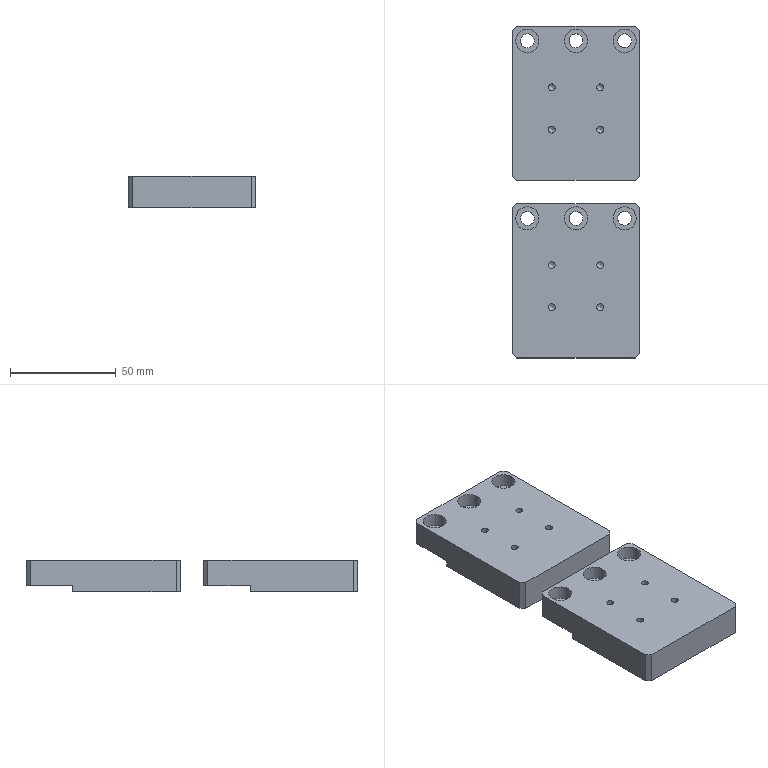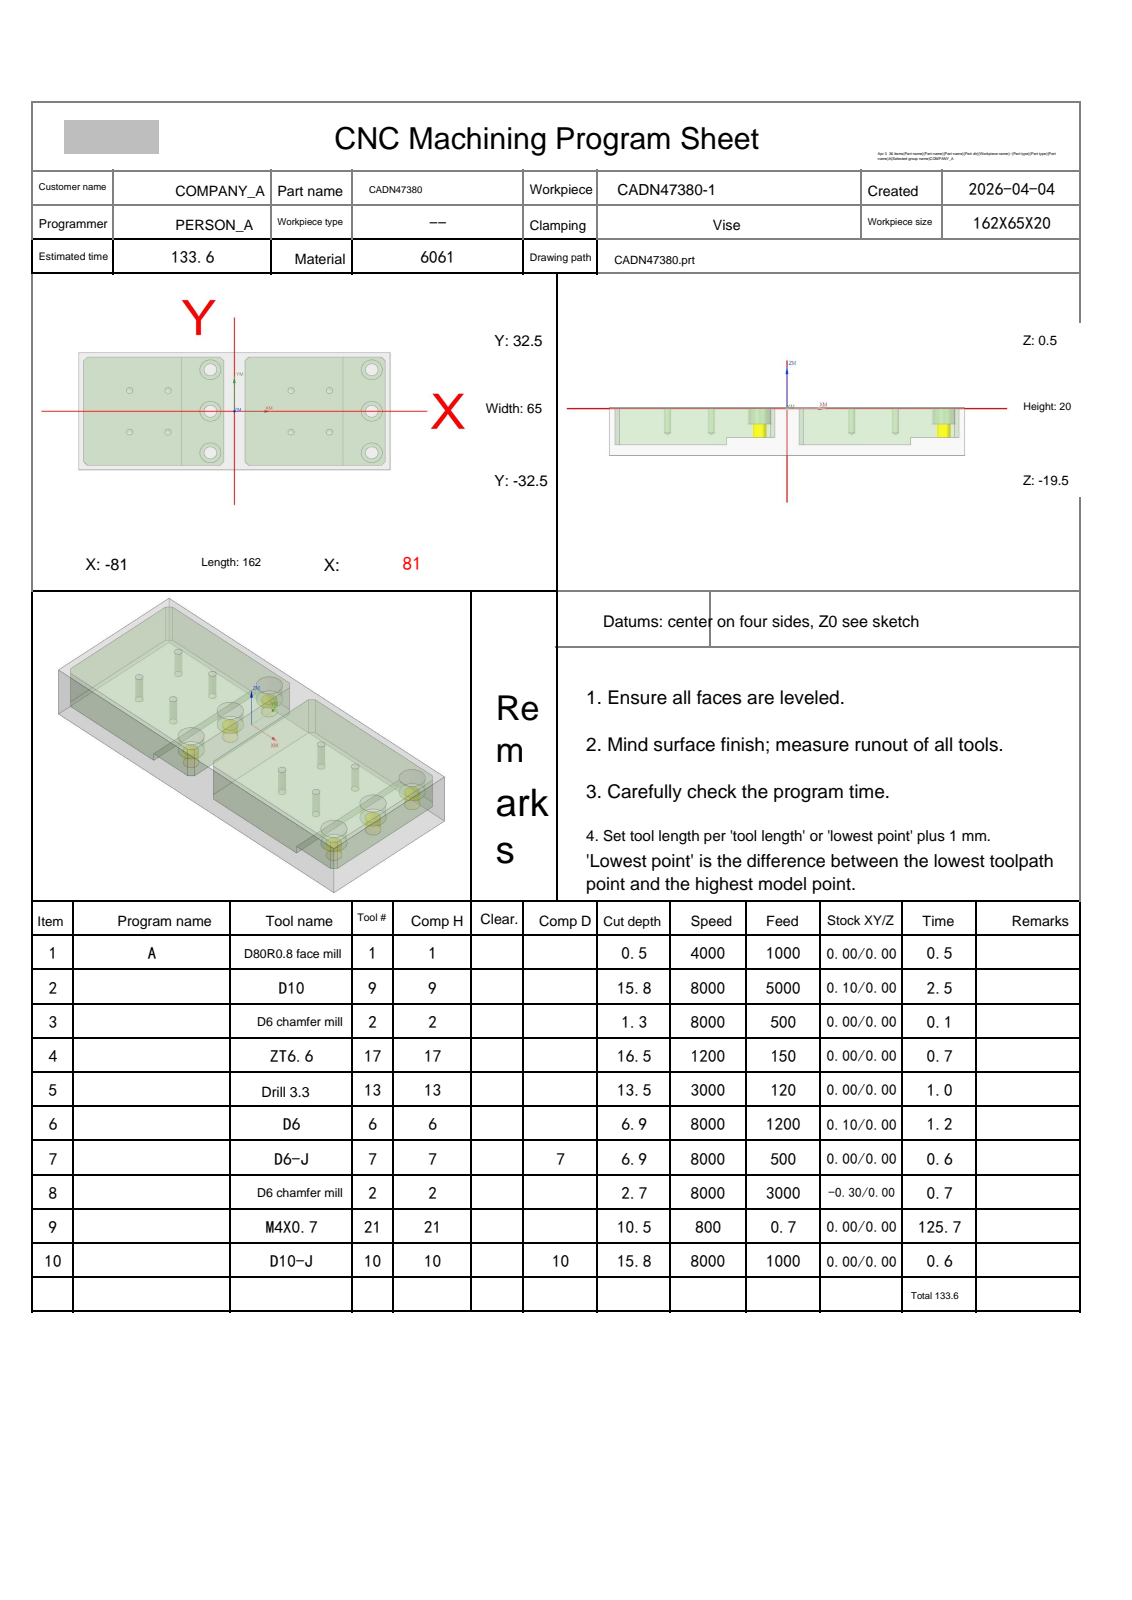NC program | NX | posted by the shop | part box 60 x 157 x 15 mm
Whole program, first 1350 of 1479 lines:
%
O0001
(Machine time: 249.80 MIN)
(===Total Tool:9===)
(T1=D80R0.8 face mill D=80.  R=0.8  D-  H01 Z=-0.   )
(T9=D10     D=10.  R=0.   D-  H09 Z=-15.3 )
(T2=D6 chamfer mill   D=6.   R=0.   D-  H02 Z=-2.2  )
(T17=ZT6.6  D=6.6  DR_a=118 D-  H17 Z=-15.98)
(T13=drill 3.3  D=3.3  DR_a=118 D-  H13 Z=-13.  )
(T6=D6      D=6.   R=0.   D-  H06 Z=-6.4  )
(T7=D6-J    D=6.   R=0.   D7  H07 Z=-6.4  )
(T21=M4X0.7 D=3.3  DR_a=180 D-  H21 Z=-10.  )
(T10=D10-J  D=10.  R=0.   D10 H10 Z=-15.3 )
G80 G90 G17 G49 G40
G91 G28 Z0
M01
N1 T01 M06
(D80R0.8 face mill  D=80. R=0.8 H=01 ce=0.00 di=0.00)
G00 G90 G54 X-123.5 Y23.333 M03 S4000
G43 H01 Z20.
M08
Z2.
G01 Z0.0 F1000.
X-118.5
X118.5
Y-23.333
X-118.5
X-123.5
Z2.
G00 Z20.
G91 G28 Z0.0
M05
M09
G91 G28 Z0.0
M01
N2 T09 M06
(D10  D=10. R=0. H=09 ce=0.10 di=0.00)
G00 G90 G54 X-42. Y35.1 M03 S8000
G43 H09 Z20.
M08
Z.5
G01 X-7.5 Z.407 F5000.
G02 X-3.894 Y33.606 Z.396 I0.0 J-5.1
G01 X-1.894 Y31.606 Z.389
G02 X-.4 Y28. Z.378 I-3.606 J-3.606
G01 Y-28. Z.227
G02 X-1.894 Y-31.606 Z.216 I-5.1 J0.0
G01 X-3.894 Y-33.606 Z.209
G02 X-7.5 Y-35.1 Z.198 I-3.606 J3.606
G01 X-76.5 Z.012
G02 X-80.106 Y-33.606 Z.001 I0.0 J5.1
G01 X-82.106 Y-31.606 Z-.006
G02 X-83.6 Y-28. Z-.017 I3.606 J3.606
G01 Y28. Z-.168
G02 X-82.106 Y31.606 Z-.179 I5.1 J0.0
G01 X-80.106 Y33.606 Z-.186
G02 X-76.5 Y35.1 Z-.197 I3.606 J-3.606
G01 X-7.5 Z-.383
G02 X-3.894 Y33.606 Z-.394 I0.0 J-5.1
G01 X-1.894 Y31.606 Z-.401
G02 X-.4 Y28. Z-.412 I-3.606 J-3.606
G01 Y-28. Z-.563
G02 X-1.894 Y-31.606 Z-.574 I-5.1 J0.0
G01 X-3.894 Y-33.606 Z-.581
G02 X-7.5 Y-35.1 Z-.592 I-3.606 J3.606
G01 X-76.5 Z-.778
G02 X-80.106 Y-33.606 Z-.789 I0.0 J5.1
G01 X-82.106 Y-31.606 Z-.796
G02 X-83.6 Y-28. Z-.807 I3.606 J3.606
G01 Y28. Z-.958
G02 X-82.106 Y31.606 Z-.969 I5.1 J0.0
G01 X-80.106 Y33.606 Z-.976
G02 X-76.5 Y35.1 Z-.987 I3.606 J-3.606
G01 X-7.5 Z-1.173
G02 X-3.894 Y33.606 Z-1.184 I0.0 J-5.1
G01 X-1.894 Y31.606 Z-1.191
G02 X-.4 Y28. Z-1.202 I-3.606 J-3.606
G01 Y-28. Z-1.353
G02 X-1.894 Y-31.606 Z-1.364 I-5.1 J0.0
G01 X-3.894 Y-33.606 Z-1.371
G02 X-7.5 Y-35.1 Z-1.382 I-3.606 J3.606
G01 X-76.5 Z-1.568
G02 X-80.106 Y-33.606 Z-1.579 I0.0 J5.1
G01 X-82.106 Y-31.606 Z-1.586
G02 X-83.6 Y-28. Z-1.597 I3.606 J3.606
G01 Y28. Z-1.748
G02 X-82.106 Y31.606 Z-1.759 I5.1 J0.0
G01 X-80.106 Y33.606 Z-1.766
G02 X-76.5 Y35.1 Z-1.777 I3.606 J-3.606
G01 X-7.5 Z-1.963
G02 X-3.894 Y33.606 Z-1.974 I0.0 J-5.1
G01 X-1.894 Y31.606 Z-1.981
G02 X-.4 Y28. Z-1.992 I-3.606 J-3.606
G01 Y-28. Z-2.143
G02 X-1.894 Y-31.606 Z-2.154 I-5.1 J0.0
G01 X-3.894 Y-33.606 Z-2.161
G02 X-7.5 Y-35.1 Z-2.172 I-3.606 J3.606
G01 X-76.5 Z-2.358
G02 X-80.106 Y-33.606 Z-2.369 I0.0 J5.1
G01 X-82.106 Y-31.606 Z-2.376
G02 X-83.6 Y-28. Z-2.387 I3.606 J3.606
G01 Y28. Z-2.538
G02 X-82.106 Y31.606 Z-2.549 I5.1 J0.0
G01 X-80.106 Y33.606 Z-2.556
G02 X-76.5 Y35.1 Z-2.567 I3.606 J-3.606
G01 X-7.5 Z-2.753
G02 X-3.894 Y33.606 Z-2.764 I0.0 J-5.1
G01 X-1.894 Y31.606 Z-2.771
G02 X-.4 Y28. Z-2.782 I-3.606 J-3.606
G01 Y-28. Z-2.933
G02 X-1.894 Y-31.606 Z-2.944 I-5.1 J0.0
G01 X-3.894 Y-33.606 Z-2.951
G02 X-7.5 Y-35.1 Z-2.962 I-3.606 J3.606
G01 X-76.5 Z-3.148
G02 X-80.106 Y-33.606 Z-3.159 I0.0 J5.1
G01 X-82.106 Y-31.606 Z-3.166
G02 X-83.6 Y-28. Z-3.177 I3.606 J3.606
G01 Y28. Z-3.328
G02 X-82.106 Y31.606 Z-3.339 I5.1 J0.0
G01 X-80.106 Y33.606 Z-3.346
G02 X-76.5 Y35.1 Z-3.357 I3.606 J-3.606
G01 X-7.5 Z-3.543
G02 X-3.894 Y33.606 Z-3.554 I0.0 J-5.1
G01 X-1.894 Y31.606 Z-3.561
G02 X-.4 Y28. Z-3.572 I-3.606 J-3.606
G01 Y-28. Z-3.723
G02 X-1.894 Y-31.606 Z-3.734 I-5.1 J0.0
G01 X-3.894 Y-33.606 Z-3.741
G02 X-7.5 Y-35.1 Z-3.752 I-3.606 J3.606
G01 X-76.5 Z-3.938
G02 X-80.106 Y-33.606 Z-3.949 I0.0 J5.1
G01 X-82.106 Y-31.606 Z-3.956
G02 X-83.6 Y-28. Z-3.967 I3.606 J3.606
G01 Y28. Z-4.118
G02 X-82.106 Y31.606 Z-4.129 I5.1 J0.0
G01 X-80.106 Y33.606 Z-4.136
G02 X-76.5 Y35.1 Z-4.147 I3.606 J-3.606
G01 X-7.5 Z-4.333
G02 X-3.894 Y33.606 Z-4.344 I0.0 J-5.1
G01 X-1.894 Y31.606 Z-4.351
G02 X-.4 Y28. Z-4.362 I-3.606 J-3.606
G01 Y-28. Z-4.513
G02 X-1.894 Y-31.606 Z-4.524 I-5.1 J0.0
G01 X-3.894 Y-33.606 Z-4.531
G02 X-7.5 Y-35.1 Z-4.542 I-3.606 J3.606
G01 X-76.5 Z-4.728
G02 X-80.106 Y-33.606 Z-4.739 I0.0 J5.1
G01 X-82.106 Y-31.606 Z-4.746
G02 X-83.6 Y-28. Z-4.757 I3.606 J3.606
G01 Y28. Z-4.908
G02 X-82.106 Y31.606 Z-4.919 I5.1 J0.0
G01 X-80.106 Y33.606 Z-4.926
G02 X-76.5 Y35.1 Z-4.937 I3.606 J-3.606
G01 X-7.5 Z-5.123
G02 X-3.894 Y33.606 Z-5.134 I0.0 J-5.1
G01 X-1.894 Y31.606 Z-5.141
G02 X-.4 Y28. Z-5.152 I-3.606 J-3.606
G01 Y-28. Z-5.303
G02 X-1.894 Y-31.606 Z-5.314 I-5.1 J0.0
G01 X-3.894 Y-33.606 Z-5.321
G02 X-7.5 Y-35.1 Z-5.332 I-3.606 J3.606
G01 X-76.5 Z-5.518
G02 X-80.106 Y-33.606 Z-5.529 I0.0 J5.1
G01 X-82.106 Y-31.606 Z-5.536
G02 X-83.6 Y-28. Z-5.547 I3.606 J3.606
G01 Y28. Z-5.698
G02 X-82.106 Y31.606 Z-5.709 I5.1 J0.0
G01 X-80.106 Y33.606 Z-5.716
G02 X-76.5 Y35.1 Z-5.727 I3.606 J-3.606
G01 X-7.5 Z-5.913
G02 X-3.894 Y33.606 Z-5.924 I0.0 J-5.1
G01 X-1.894 Y31.606 Z-5.931
G02 X-.4 Y28. Z-5.942 I-3.606 J-3.606
G01 Y-28. Z-6.093
G02 X-1.894 Y-31.606 Z-6.104 I-5.1 J0.0
G01 X-3.894 Y-33.606 Z-6.111
G02 X-7.5 Y-35.1 Z-6.122 I-3.606 J3.606
G01 X-76.5 Z-6.308
G02 X-80.106 Y-33.606 Z-6.319 I0.0 J5.1
G01 X-82.106 Y-31.606 Z-6.326
G02 X-83.6 Y-28. Z-6.337 I3.606 J3.606
G01 Y28. Z-6.488
G02 X-82.106 Y31.606 Z-6.499 I5.1 J0.0
G01 X-80.106 Y33.606 Z-6.506
G02 X-76.5 Y35.1 Z-6.517 I3.606 J-3.606
G01 X-7.5 Z-6.703
G02 X-3.894 Y33.606 Z-6.714 I0.0 J-5.1
G01 X-1.894 Y31.606 Z-6.721
G02 X-.4 Y28. Z-6.732 I-3.606 J-3.606
G01 Y-28. Z-6.883
G02 X-1.894 Y-31.606 Z-6.894 I-5.1 J0.0
G01 X-3.894 Y-33.606 Z-6.901
G02 X-7.5 Y-35.1 Z-6.912 I-3.606 J3.606
G01 X-76.5 Z-7.098
G02 X-80.106 Y-33.606 Z-7.109 I0.0 J5.1
G01 X-82.106 Y-31.606 Z-7.116
G02 X-83.6 Y-28. Z-7.127 I3.606 J3.606
G01 Y28. Z-7.278
G02 X-82.106 Y31.606 Z-7.289 I5.1 J0.0
G01 X-80.106 Y33.606 Z-7.296
G02 X-76.5 Y35.1 Z-7.307 I3.606 J-3.606
G01 X-7.5 Z-7.493
G02 X-3.894 Y33.606 Z-7.504 I0.0 J-5.1
G01 X-1.894 Y31.606 Z-7.511
G02 X-.4 Y28. Z-7.522 I-3.606 J-3.606
G01 Y-28. Z-7.673
G02 X-1.894 Y-31.606 Z-7.684 I-5.1 J0.0
G01 X-3.894 Y-33.606 Z-7.691
G02 X-7.5 Y-35.1 Z-7.702 I-3.606 J3.606
G01 X-76.5 Z-7.888
G02 X-80.106 Y-33.606 Z-7.899 I0.0 J5.1
G01 X-82.106 Y-31.606 Z-7.906
G02 X-83.6 Y-28. Z-7.917 I3.606 J3.606
G01 Y28. Z-8.068
G02 X-82.106 Y31.606 Z-8.079 I5.1 J0.0
G01 X-80.106 Y33.606 Z-8.086
G02 X-76.5 Y35.1 Z-8.097 I3.606 J-3.606
G01 X-7.5 Z-8.283
G02 X-3.894 Y33.606 Z-8.294 I0.0 J-5.1
G01 X-1.894 Y31.606 Z-8.301
G02 X-.4 Y28. Z-8.312 I-3.606 J-3.606
G01 Y-28. Z-8.463
G02 X-1.894 Y-31.606 Z-8.474 I-5.1 J0.0
G01 X-3.894 Y-33.606 Z-8.481
G02 X-7.5 Y-35.1 Z-8.492 I-3.606 J3.606
G01 X-76.5 Z-8.678
G02 X-80.106 Y-33.606 Z-8.689 I0.0 J5.1
G01 X-82.106 Y-31.606 Z-8.696
G02 X-83.6 Y-28. Z-8.707 I3.606 J3.606
G01 Y28. Z-8.858
G02 X-82.106 Y31.606 Z-8.869 I5.1 J0.0
G01 X-80.106 Y33.606 Z-8.876
G02 X-76.5 Y35.1 Z-8.887 I3.606 J-3.606
G01 X-7.5 Z-9.073
G02 X-3.894 Y33.606 Z-9.084 I0.0 J-5.1
G01 X-1.894 Y31.606 Z-9.091
G02 X-.4 Y28. Z-9.102 I-3.606 J-3.606
G01 Y-28. Z-9.253
G02 X-1.894 Y-31.606 Z-9.264 I-5.1 J0.0
G01 X-3.894 Y-33.606 Z-9.271
G02 X-7.5 Y-35.1 Z-9.282 I-3.606 J3.606
G01 X-76.5 Z-9.468
G02 X-80.106 Y-33.606 Z-9.479 I0.0 J5.1
G01 X-82.106 Y-31.606 Z-9.486
G02 X-83.6 Y-28. Z-9.497 I3.606 J3.606
G01 Y28. Z-9.648
G02 X-82.106 Y31.606 Z-9.659 I5.1 J0.0
G01 X-80.106 Y33.606 Z-9.666
G02 X-76.5 Y35.1 Z-9.677 I3.606 J-3.606
G01 X-7.5 Z-9.863
G02 X-3.894 Y33.606 Z-9.874 I0.0 J-5.1
G01 X-1.894 Y31.606 Z-9.881
G02 X-.4 Y28. Z-9.892 I-3.606 J-3.606
G01 Y-28. Z-10.043
G02 X-1.894 Y-31.606 Z-10.054 I-5.1 J0.0
G01 X-3.894 Y-33.606 Z-10.061
G02 X-7.5 Y-35.1 Z-10.072 I-3.606 J3.606
G01 X-76.5 Z-10.258
G02 X-80.106 Y-33.606 Z-10.269 I0.0 J5.1
G01 X-82.106 Y-31.606 Z-10.276
G02 X-83.6 Y-28. Z-10.287 I3.606 J3.606
G01 Y28. Z-10.438
G02 X-82.106 Y31.606 Z-10.449 I5.1 J0.0
G01 X-80.106 Y33.606 Z-10.456
G02 X-76.5 Y35.1 Z-10.467 I3.606 J-3.606
G01 X-7.5 Z-10.653
G02 X-3.894 Y33.606 Z-10.664 I0.0 J-5.1
G01 X-1.894 Y31.606 Z-10.671
G02 X-.4 Y28. Z-10.682 I-3.606 J-3.606
G01 Y-28. Z-10.833
G02 X-1.894 Y-31.606 Z-10.844 I-5.1 J0.0
G01 X-3.894 Y-33.606 Z-10.851
G02 X-7.5 Y-35.1 Z-10.862 I-3.606 J3.606
G01 X-76.5 Z-11.048
G02 X-80.106 Y-33.606 Z-11.059 I0.0 J5.1
G01 X-82.106 Y-31.606 Z-11.066
G02 X-83.6 Y-28. Z-11.077 I3.606 J3.606
G01 Y28. Z-11.228
G02 X-82.106 Y31.606 Z-11.239 I5.1 J0.0
G01 X-80.106 Y33.606 Z-11.246
G02 X-76.5 Y35.1 Z-11.257 I3.606 J-3.606
G01 X-7.5 Z-11.443
G02 X-3.894 Y33.606 Z-11.454 I0.0 J-5.1
G01 X-1.894 Y31.606 Z-11.461
G02 X-.4 Y28. Z-11.472 I-3.606 J-3.606
G01 Y-28. Z-11.623
G02 X-1.894 Y-31.606 Z-11.634 I-5.1 J0.0
G01 X-3.894 Y-33.606 Z-11.641
G02 X-7.5 Y-35.1 Z-11.652 I-3.606 J3.606
G01 X-76.5 Z-11.838
G02 X-80.106 Y-33.606 Z-11.849 I0.0 J5.1
G01 X-82.106 Y-31.606 Z-11.856
G02 X-83.6 Y-28. Z-11.867 I3.606 J3.606
G01 Y28. Z-12.018
G02 X-82.106 Y31.606 Z-12.029 I5.1 J0.0
G01 X-80.106 Y33.606 Z-12.036
G02 X-76.5 Y35.1 Z-12.047 I3.606 J-3.606
G01 X-7.5 Z-12.233
G02 X-3.894 Y33.606 Z-12.244 I0.0 J-5.1
G01 X-1.894 Y31.606 Z-12.251
G02 X-.4 Y28. Z-12.262 I-3.606 J-3.606
G01 Y-28. Z-12.413
G02 X-1.894 Y-31.606 Z-12.424 I-5.1 J0.0
G01 X-3.894 Y-33.606 Z-12.431
G02 X-7.5 Y-35.1 Z-12.442 I-3.606 J3.606
G01 X-76.5 Z-12.628
G02 X-80.106 Y-33.606 Z-12.639 I0.0 J5.1
G01 X-82.106 Y-31.606 Z-12.646
G02 X-83.6 Y-28. Z-12.657 I3.606 J3.606
G01 Y28. Z-12.808
G02 X-82.106 Y31.606 Z-12.819 I5.1 J0.0
G01 X-80.106 Y33.606 Z-12.826
G02 X-76.5 Y35.1 Z-12.837 I3.606 J-3.606
G01 X-7.5 Z-13.023
G02 X-3.894 Y33.606 Z-13.034 I0.0 J-5.1
G01 X-1.894 Y31.606 Z-13.041
G02 X-.4 Y28. Z-13.052 I-3.606 J-3.606
G01 Y-28. Z-13.203
G02 X-1.894 Y-31.606 Z-13.214 I-5.1 J0.0
G01 X-3.894 Y-33.606 Z-13.221
G02 X-7.5 Y-35.1 Z-13.232 I-3.606 J3.606
G01 X-76.5 Z-13.418
G02 X-80.106 Y-33.606 Z-13.429 I0.0 J5.1
G01 X-82.106 Y-31.606 Z-13.436
G02 X-83.6 Y-28. Z-13.447 I3.606 J3.606
G01 Y28. Z-13.598
G02 X-82.106 Y31.606 Z-13.609 I5.1 J0.0
G01 X-80.106 Y33.606 Z-13.616
G02 X-76.5 Y35.1 Z-13.627 I3.606 J-3.606
G01 X-7.5 Z-13.813
G02 X-3.894 Y33.606 Z-13.824 I0.0 J-5.1
G01 X-1.894 Y31.606 Z-13.831
G02 X-.4 Y28. Z-13.842 I-3.606 J-3.606
G01 Y-28. Z-13.993
G02 X-1.894 Y-31.606 Z-14.004 I-5.1 J0.0
G01 X-3.894 Y-33.606 Z-14.011
G02 X-7.5 Y-35.1 Z-14.022 I-3.606 J3.606
G01 X-76.5 Z-14.208
G02 X-80.106 Y-33.606 Z-14.219 I0.0 J5.1
G01 X-82.106 Y-31.606 Z-14.226
G02 X-83.6 Y-28. Z-14.237 I3.606 J3.606
G01 Y28. Z-14.388
G02 X-82.106 Y31.606 Z-14.399 I5.1 J0.0
G01 X-80.106 Y33.606 Z-14.406
G02 X-76.5 Y35.1 Z-14.417 I3.606 J-3.606
G01 X-7.5 Z-14.603
G02 X-3.894 Y33.606 Z-14.614 I0.0 J-5.1
G01 X-1.894 Y31.606 Z-14.621
G02 X-.4 Y28. Z-14.632 I-3.606 J-3.606
G01 Y-28. Z-14.783
G02 X-1.894 Y-31.606 Z-14.794 I-5.1 J0.0
G01 X-3.894 Y-33.606 Z-14.801
G02 X-7.5 Y-35.1 Z-14.812 I-3.606 J3.606
G01 X-76.5 Z-14.998
G02 X-80.106 Y-33.606 Z-15.009 I0.0 J5.1
G01 X-82.106 Y-31.606 Z-15.016
G02 X-83.6 Y-28. Z-15.027 I3.606 J3.606
G01 Y28. Z-15.178
G02 X-82.106 Y31.606 Z-15.189 I5.1 J0.0
G01 X-80.106 Y33.606 Z-15.196
G02 X-76.5 Y35.1 Z-15.207 I3.606 J-3.606
G01 X-42. Z-15.3
X-7.5
G02 X-3.894 Y33.606 I0.0 J-5.1
G01 X-1.894 Y31.606
G02 X-.4 Y28. I-3.606 J-3.606
G01 Y-28.
G02 X-1.894 Y-31.606 I-5.1 J0.0
G01 X-3.894 Y-33.606
G02 X-7.5 Y-35.1 I-3.606 J3.606
G01 X-76.5
G02 X-80.106 Y-33.606 I0.0 J5.1
G01 X-82.106 Y-31.606
G02 X-83.6 Y-28. I3.606 J3.606
G01 Y28.
G02 X-82.106 Y31.606 I5.1 J0.0
G01 X-80.106 Y33.606
G02 X-76.5 Y35.1 I3.606 J-3.606
G01 X-42.
X-41.5
Z-14.3
G00 Z20.
X42.
Z.5
G01 X76.5 Z.407
G02 X80.106 Y33.606 Z.396 I0.0 J-5.1
G01 X82.106 Y31.606 Z.389
G02 X83.6 Y28. Z.378 I-3.606 J-3.606
G01 Y-28. Z.227
G02 X82.106 Y-31.606 Z.216 I-5.1 J0.0
G01 X80.106 Y-33.606 Z.209
G02 X76.5 Y-35.1 Z.198 I-3.606 J3.606
G01 X7.5 Z.012
G02 X3.894 Y-33.606 Z.001 I0.0 J5.1
G01 X1.894 Y-31.606 Z-.006
G02 X.4 Y-28. Z-.017 I3.606 J3.606
G01 Y28. Z-.168
G02 X1.894 Y31.606 Z-.179 I5.1 J0.0
G01 X3.894 Y33.606 Z-.186
G02 X7.5 Y35.1 Z-.197 I3.606 J-3.606
G01 X76.5 Z-.383
G02 X80.106 Y33.606 Z-.394 I0.0 J-5.1
G01 X82.106 Y31.606 Z-.401
G02 X83.6 Y28. Z-.412 I-3.606 J-3.606
G01 Y-28. Z-.563
G02 X82.106 Y-31.606 Z-.574 I-5.1 J0.0
G01 X80.106 Y-33.606 Z-.581
G02 X76.5 Y-35.1 Z-.592 I-3.606 J3.606
G01 X7.5 Z-.778
G02 X3.894 Y-33.606 Z-.789 I0.0 J5.1
G01 X1.894 Y-31.606 Z-.796
G02 X.4 Y-28. Z-.807 I3.606 J3.606
G01 Y28. Z-.958
G02 X1.894 Y31.606 Z-.969 I5.1 J0.0
G01 X3.894 Y33.606 Z-.976
G02 X7.5 Y35.1 Z-.987 I3.606 J-3.606
G01 X76.5 Z-1.173
G02 X80.106 Y33.606 Z-1.184 I0.0 J-5.1
G01 X82.106 Y31.606 Z-1.191
G02 X83.6 Y28. Z-1.202 I-3.606 J-3.606
G01 Y-28. Z-1.353
G02 X82.106 Y-31.606 Z-1.364 I-5.1 J0.0
G01 X80.106 Y-33.606 Z-1.371
G02 X76.5 Y-35.1 Z-1.382 I-3.606 J3.606
G01 X7.5 Z-1.568
G02 X3.894 Y-33.606 Z-1.579 I0.0 J5.1
G01 X1.894 Y-31.606 Z-1.586
G02 X.4 Y-28. Z-1.597 I3.606 J3.606
G01 Y28. Z-1.748
G02 X1.894 Y31.606 Z-1.759 I5.1 J0.0
G01 X3.894 Y33.606 Z-1.766
G02 X7.5 Y35.1 Z-1.777 I3.606 J-3.606
G01 X76.5 Z-1.963
G02 X80.106 Y33.606 Z-1.974 I0.0 J-5.1
G01 X82.106 Y31.606 Z-1.981
G02 X83.6 Y28. Z-1.992 I-3.606 J-3.606
G01 Y-28. Z-2.143
G02 X82.106 Y-31.606 Z-2.154 I-5.1 J0.0
G01 X80.106 Y-33.606 Z-2.161
G02 X76.5 Y-35.1 Z-2.172 I-3.606 J3.606
G01 X7.5 Z-2.358
G02 X3.894 Y-33.606 Z-2.369 I0.0 J5.1
G01 X1.894 Y-31.606 Z-2.376
G02 X.4 Y-28. Z-2.387 I3.606 J3.606
G01 Y28. Z-2.538
G02 X1.894 Y31.606 Z-2.549 I5.1 J0.0
G01 X3.894 Y33.606 Z-2.556
G02 X7.5 Y35.1 Z-2.567 I3.606 J-3.606
G01 X76.5 Z-2.753
G02 X80.106 Y33.606 Z-2.764 I0.0 J-5.1
G01 X82.106 Y31.606 Z-2.771
G02 X83.6 Y28. Z-2.782 I-3.606 J-3.606
G01 Y-28. Z-2.933
G02 X82.106 Y-31.606 Z-2.944 I-5.1 J0.0
G01 X80.106 Y-33.606 Z-2.951
G02 X76.5 Y-35.1 Z-2.962 I-3.606 J3.606
G01 X7.5 Z-3.148
G02 X3.894 Y-33.606 Z-3.159 I0.0 J5.1
G01 X1.894 Y-31.606 Z-3.166
G02 X.4 Y-28. Z-3.177 I3.606 J3.606
G01 Y28. Z-3.328
G02 X1.894 Y31.606 Z-3.339 I5.1 J0.0
G01 X3.894 Y33.606 Z-3.346
G02 X7.5 Y35.1 Z-3.357 I3.606 J-3.606
G01 X76.5 Z-3.543
G02 X80.106 Y33.606 Z-3.554 I0.0 J-5.1
G01 X82.106 Y31.606 Z-3.561
G02 X83.6 Y28. Z-3.572 I-3.606 J-3.606
G01 Y-28. Z-3.723
G02 X82.106 Y-31.606 Z-3.734 I-5.1 J0.0
G01 X80.106 Y-33.606 Z-3.741
G02 X76.5 Y-35.1 Z-3.752 I-3.606 J3.606
G01 X7.5 Z-3.938
G02 X3.894 Y-33.606 Z-3.949 I0.0 J5.1
G01 X1.894 Y-31.606 Z-3.956
G02 X.4 Y-28. Z-3.967 I3.606 J3.606
G01 Y28. Z-4.118
G02 X1.894 Y31.606 Z-4.129 I5.1 J0.0
G01 X3.894 Y33.606 Z-4.136
G02 X7.5 Y35.1 Z-4.147 I3.606 J-3.606
G01 X76.5 Z-4.333
G02 X80.106 Y33.606 Z-4.344 I0.0 J-5.1
G01 X82.106 Y31.606 Z-4.351
G02 X83.6 Y28. Z-4.362 I-3.606 J-3.606
G01 Y-28. Z-4.513
G02 X82.106 Y-31.606 Z-4.524 I-5.1 J0.0
G01 X80.106 Y-33.606 Z-4.531
G02 X76.5 Y-35.1 Z-4.542 I-3.606 J3.606
G01 X7.5 Z-4.728
G02 X3.894 Y-33.606 Z-4.739 I0.0 J5.1
G01 X1.894 Y-31.606 Z-4.746
G02 X.4 Y-28. Z-4.757 I3.606 J3.606
G01 Y28. Z-4.908
G02 X1.894 Y31.606 Z-4.919 I5.1 J0.0
G01 X3.894 Y33.606 Z-4.926
G02 X7.5 Y35.1 Z-4.937 I3.606 J-3.606
G01 X76.5 Z-5.123
G02 X80.106 Y33.606 Z-5.134 I0.0 J-5.1
G01 X82.106 Y31.606 Z-5.141
G02 X83.6 Y28. Z-5.152 I-3.606 J-3.606
G01 Y-28. Z-5.303
G02 X82.106 Y-31.606 Z-5.314 I-5.1 J0.0
G01 X80.106 Y-33.606 Z-5.321
G02 X76.5 Y-35.1 Z-5.332 I-3.606 J3.606
G01 X7.5 Z-5.518
G02 X3.894 Y-33.606 Z-5.529 I0.0 J5.1
G01 X1.894 Y-31.606 Z-5.536
G02 X.4 Y-28. Z-5.547 I3.606 J3.606
G01 Y28. Z-5.698
G02 X1.894 Y31.606 Z-5.709 I5.1 J0.0
G01 X3.894 Y33.606 Z-5.716
G02 X7.5 Y35.1 Z-5.727 I3.606 J-3.606
G01 X76.5 Z-5.913
G02 X80.106 Y33.606 Z-5.924 I0.0 J-5.1
G01 X82.106 Y31.606 Z-5.931
G02 X83.6 Y28. Z-5.942 I-3.606 J-3.606
G01 Y-28. Z-6.093
G02 X82.106 Y-31.606 Z-6.104 I-5.1 J0.0
G01 X80.106 Y-33.606 Z-6.111
G02 X76.5 Y-35.1 Z-6.122 I-3.606 J3.606
G01 X7.5 Z-6.308
G02 X3.894 Y-33.606 Z-6.319 I0.0 J5.1
G01 X1.894 Y-31.606 Z-6.326
G02 X.4 Y-28. Z-6.337 I3.606 J3.606
G01 Y28. Z-6.488
G02 X1.894 Y31.606 Z-6.499 I5.1 J0.0
G01 X3.894 Y33.606 Z-6.506
G02 X7.5 Y35.1 Z-6.517 I3.606 J-3.606
G01 X76.5 Z-6.703
G02 X80.106 Y33.606 Z-6.714 I0.0 J-5.1
G01 X82.106 Y31.606 Z-6.721
G02 X83.6 Y28. Z-6.732 I-3.606 J-3.606
G01 Y-28. Z-6.883
G02 X82.106 Y-31.606 Z-6.894 I-5.1 J0.0
G01 X80.106 Y-33.606 Z-6.901
G02 X76.5 Y-35.1 Z-6.912 I-3.606 J3.606
G01 X7.5 Z-7.098
G02 X3.894 Y-33.606 Z-7.109 I0.0 J5.1
G01 X1.894 Y-31.606 Z-7.116
G02 X.4 Y-28. Z-7.127 I3.606 J3.606
G01 Y28. Z-7.278
G02 X1.894 Y31.606 Z-7.289 I5.1 J0.0
G01 X3.894 Y33.606 Z-7.296
G02 X7.5 Y35.1 Z-7.307 I3.606 J-3.606
G01 X76.5 Z-7.493
G02 X80.106 Y33.606 Z-7.504 I0.0 J-5.1
G01 X82.106 Y31.606 Z-7.511
G02 X83.6 Y28. Z-7.522 I-3.606 J-3.606
G01 Y-28. Z-7.673
G02 X82.106 Y-31.606 Z-7.684 I-5.1 J0.0
G01 X80.106 Y-33.606 Z-7.691
G02 X76.5 Y-35.1 Z-7.702 I-3.606 J3.606
G01 X7.5 Z-7.888
G02 X3.894 Y-33.606 Z-7.899 I0.0 J5.1
G01 X1.894 Y-31.606 Z-7.906
G02 X.4 Y-28. Z-7.917 I3.606 J3.606
G01 Y28. Z-8.068
G02 X1.894 Y31.606 Z-8.079 I5.1 J0.0
G01 X3.894 Y33.606 Z-8.086
G02 X7.5 Y35.1 Z-8.097 I3.606 J-3.606
G01 X76.5 Z-8.283
G02 X80.106 Y33.606 Z-8.294 I0.0 J-5.1
G01 X82.106 Y31.606 Z-8.301
G02 X83.6 Y28. Z-8.312 I-3.606 J-3.606
G01 Y-28. Z-8.463
G02 X82.106 Y-31.606 Z-8.474 I-5.1 J0.0
G01 X80.106 Y-33.606 Z-8.481
G02 X76.5 Y-35.1 Z-8.492 I-3.606 J3.606
G01 X7.5 Z-8.678
G02 X3.894 Y-33.606 Z-8.689 I0.0 J5.1
G01 X1.894 Y-31.606 Z-8.696
G02 X.4 Y-28. Z-8.707 I3.606 J3.606
G01 Y28. Z-8.858
G02 X1.894 Y31.606 Z-8.869 I5.1 J0.0
G01 X3.894 Y33.606 Z-8.876
G02 X7.5 Y35.1 Z-8.887 I3.606 J-3.606
G01 X76.5 Z-9.073
G02 X80.106 Y33.606 Z-9.084 I0.0 J-5.1
G01 X82.106 Y31.606 Z-9.091
G02 X83.6 Y28. Z-9.102 I-3.606 J-3.606
G01 Y-28. Z-9.253
G02 X82.106 Y-31.606 Z-9.264 I-5.1 J0.0
G01 X80.106 Y-33.606 Z-9.271
G02 X76.5 Y-35.1 Z-9.282 I-3.606 J3.606
G01 X7.5 Z-9.468
G02 X3.894 Y-33.606 Z-9.479 I0.0 J5.1
G01 X1.894 Y-31.606 Z-9.486
G02 X.4 Y-28. Z-9.497 I3.606 J3.606
G01 Y28. Z-9.648
G02 X1.894 Y31.606 Z-9.659 I5.1 J0.0
G01 X3.894 Y33.606 Z-9.666
G02 X7.5 Y35.1 Z-9.677 I3.606 J-3.606
G01 X76.5 Z-9.863
G02 X80.106 Y33.606 Z-9.874 I0.0 J-5.1
G01 X82.106 Y31.606 Z-9.881
G02 X83.6 Y28. Z-9.892 I-3.606 J-3.606
G01 Y-28. Z-10.043
G02 X82.106 Y-31.606 Z-10.054 I-5.1 J0.0
G01 X80.106 Y-33.606 Z-10.061
G02 X76.5 Y-35.1 Z-10.072 I-3.606 J3.606
G01 X7.5 Z-10.258
G02 X3.894 Y-33.606 Z-10.269 I0.0 J5.1
G01 X1.894 Y-31.606 Z-10.276
G02 X.4 Y-28. Z-10.287 I3.606 J3.606
G01 Y28. Z-10.438
G02 X1.894 Y31.606 Z-10.449 I5.1 J0.0
G01 X3.894 Y33.606 Z-10.456
G02 X7.5 Y35.1 Z-10.467 I3.606 J-3.606
G01 X76.5 Z-10.653
G02 X80.106 Y33.606 Z-10.664 I0.0 J-5.1
G01 X82.106 Y31.606 Z-10.671
G02 X83.6 Y28. Z-10.682 I-3.606 J-3.606
G01 Y-28. Z-10.833
G02 X82.106 Y-31.606 Z-10.844 I-5.1 J0.0
G01 X80.106 Y-33.606 Z-10.851
G02 X76.5 Y-35.1 Z-10.862 I-3.606 J3.606
G01 X7.5 Z-11.048
G02 X3.894 Y-33.606 Z-11.059 I0.0 J5.1
G01 X1.894 Y-31.606 Z-11.066
G02 X.4 Y-28. Z-11.077 I3.606 J3.606
G01 Y28. Z-11.228
G02 X1.894 Y31.606 Z-11.239 I5.1 J0.0
G01 X3.894 Y33.606 Z-11.246
G02 X7.5 Y35.1 Z-11.257 I3.606 J-3.606
G01 X76.5 Z-11.443
G02 X80.106 Y33.606 Z-11.454 I0.0 J-5.1
G01 X82.106 Y31.606 Z-11.461
G02 X83.6 Y28. Z-11.472 I-3.606 J-3.606
G01 Y-28. Z-11.623
G02 X82.106 Y-31.606 Z-11.634 I-5.1 J0.0
G01 X80.106 Y-33.606 Z-11.641
G02 X76.5 Y-35.1 Z-11.652 I-3.606 J3.606
G01 X7.5 Z-11.838
G02 X3.894 Y-33.606 Z-11.849 I0.0 J5.1
G01 X1.894 Y-31.606 Z-11.856
G02 X.4 Y-28. Z-11.867 I3.606 J3.606
G01 Y28. Z-12.018
G02 X1.894 Y31.606 Z-12.029 I5.1 J0.0
G01 X3.894 Y33.606 Z-12.036
G02 X7.5 Y35.1 Z-12.047 I3.606 J-3.606
G01 X76.5 Z-12.233
G02 X80.106 Y33.606 Z-12.244 I0.0 J-5.1
G01 X82.106 Y31.606 Z-12.251
G02 X83.6 Y28. Z-12.262 I-3.606 J-3.606
G01 Y-28. Z-12.413
G02 X82.106 Y-31.606 Z-12.424 I-5.1 J0.0
G01 X80.106 Y-33.606 Z-12.431
G02 X76.5 Y-35.1 Z-12.442 I-3.606 J3.606
G01 X7.5 Z-12.628
G02 X3.894 Y-33.606 Z-12.639 I0.0 J5.1
G01 X1.894 Y-31.606 Z-12.646
G02 X.4 Y-28. Z-12.657 I3.606 J3.606
G01 Y28. Z-12.808
G02 X1.894 Y31.606 Z-12.819 I5.1 J0.0
G01 X3.894 Y33.606 Z-12.826
G02 X7.5 Y35.1 Z-12.837 I3.606 J-3.606
G01 X76.5 Z-13.023
G02 X80.106 Y33.606 Z-13.034 I0.0 J-5.1
G01 X82.106 Y31.606 Z-13.041
G02 X83.6 Y28. Z-13.052 I-3.606 J-3.606
G01 Y-28. Z-13.203
G02 X82.106 Y-31.606 Z-13.214 I-5.1 J0.0
G01 X80.106 Y-33.606 Z-13.221
G02 X76.5 Y-35.1 Z-13.232 I-3.606 J3.606
G01 X7.5 Z-13.418
G02 X3.894 Y-33.606 Z-13.429 I0.0 J5.1
G01 X1.894 Y-31.606 Z-13.436
G02 X.4 Y-28. Z-13.447 I3.606 J3.606
G01 Y28. Z-13.598
G02 X1.894 Y31.606 Z-13.609 I5.1 J0.0
G01 X3.894 Y33.606 Z-13.616
G02 X7.5 Y35.1 Z-13.627 I3.606 J-3.606
G01 X76.5 Z-13.813
G02 X80.106 Y33.606 Z-13.824 I0.0 J-5.1
G01 X82.106 Y31.606 Z-13.831
G02 X83.6 Y28. Z-13.842 I-3.606 J-3.606
G01 Y-28. Z-13.993
G02 X82.106 Y-31.606 Z-14.004 I-5.1 J0.0
G01 X80.106 Y-33.606 Z-14.011
G02 X76.5 Y-35.1 Z-14.022 I-3.606 J3.606
G01 X7.5 Z-14.208
G02 X3.894 Y-33.606 Z-14.219 I0.0 J5.1
G01 X1.894 Y-31.606 Z-14.226
G02 X.4 Y-28. Z-14.237 I3.606 J3.606
G01 Y28. Z-14.388
G02 X1.894 Y31.606 Z-14.399 I5.1 J0.0
G01 X3.894 Y33.606 Z-14.406
G02 X7.5 Y35.1 Z-14.417 I3.606 J-3.606
G01 X76.5 Z-14.603
G02 X80.106 Y33.606 Z-14.614 I0.0 J-5.1
G01 X82.106 Y31.606 Z-14.621
G02 X83.6 Y28. Z-14.632 I-3.606 J-3.606
G01 Y-28. Z-14.783
G02 X82.106 Y-31.606 Z-14.794 I-5.1 J0.0
G01 X80.106 Y-33.606 Z-14.801
G02 X76.5 Y-35.1 Z-14.812 I-3.606 J3.606
G01 X7.5 Z-14.998
G02 X3.894 Y-33.606 Z-15.009 I0.0 J5.1
G01 X1.894 Y-31.606 Z-15.016
G02 X.4 Y-28. Z-15.027 I3.606 J3.606
G01 Y28. Z-15.178
G02 X1.894 Y31.606 Z-15.189 I5.1 J0.0
G01 X3.894 Y33.606 Z-15.196
G02 X7.5 Y35.1 Z-15.207 I3.606 J-3.606
G01 X42. Z-15.3
X76.5
G02 X80.106 Y33.606 I0.0 J-5.1
G01 X82.106 Y31.606
G02 X83.6 Y28. I-3.606 J-3.606
G01 Y-28.
G02 X82.106 Y-31.606 I-5.1 J0.0
G01 X80.106 Y-33.606
G02 X76.5 Y-35.1 I-3.606 J3.606
G01 X7.5
G02 X3.894 Y-33.606 I0.0 J5.1
G01 X1.894 Y-31.606
G02 X.4 Y-28. I3.606 J3.606
G01 Y28.
G02 X1.894 Y31.606 I5.1 J0.0
G01 X3.894 Y33.606
G02 X7.5 Y35.1 I3.606 J-3.606
G01 X42.
X42.5
Z-14.3
G00 Z20.
G91 G28 Z0.0
M05
M09
G91 G28 Z0.0
M01
N3 T02 M06
(D6 chamfer mill  D=6. R=0. H=02 ce=0.00 di=0.00)
G00 G90 G54 X29.5 Y-11.5 M03 S8000
G43 H02 Z20.
M08
G98 G81 X29.5 Y-11.5 Z-.8 R1. F500.
X49.5
X71.5 Y-23.
Y0.0
Y23.
X49.5 Y11.5
X29.5
X-12.5 Y23.
Y0.0
Y-23.
X-34.5 Y-11.5
X-54.5
Y11.5
X-34.5
G80
G00 Z20.
G91 G28 Z0.0
M05
M09
G91 G28 Z0.0
M01
N4 T17 M06
(ZT6.6 D=6.6 DR_a=118 H=17)
G00 G90 G54 X-12.5 Y23. M03 S1200
G43 H17 Z20.
M08
G98 G83 X-12.5 Y23. Z-15.983 R1. F150. Q2.
Y0.0
Y-23.
X71.5
Y0.0
Y23.
G80
G00 Z20.
G91 G28 Z0.0
M05
M09
G91 G28 Z0.0
M01
N5 T13 M06
(drill 3.3 D=3.3 DR_a=118 H=13)
G00 G90 G54 X-34.5 Y11.5 M03 S3000
G43 H13 Z20.
M08
G98 G83 X-34.5 Y11.5 Z-13. R1. F120. Q2.
X-54.5
Y-11.5
X-34.5
X29.5
X49.5
Y11.5
X29.5
G80
G00 Z20.
G91 G28 Z0.0
M05
M09
G91 G28 Z0.0
M01
N6 T06 M06
(D6  D=6. R=0. H=06 ce=0.10 di=0.00)
G00 G90 G54 X-12.5 Y0.0 M03 S8000
G43 H06 Z20.
M08
Z.5
G03 X-13.7 Y-1.2 I0.0 J-1.2 F1200.
X-12.5 Y-2.4 I1.2 J0.0
X-12.5 Y-2.4 Z0.0 I0.0 J2.4
X-12.5 Y-2.4 Z-.5 I0.0 J2.4
X-12.5 Y-2.4 Z-1. I0.0 J2.4
X-12.5 Y-2.4 Z-1.5 I0.0 J2.4
X-12.5 Y-2.4 Z-2. I0.0 J2.4
X-12.5 Y-2.4 Z-2.5 I0.0 J2.4
X-12.5 Y-2.4 Z-3. I0.0 J2.4
X-12.5 Y-2.4 Z-3.5 I0.0 J2.4
X-12.5 Y-2.4 Z-4. I0.0 J2.4
X-12.5 Y-2.4 Z-4.5 I0.0 J2.4
X-12.5 Y-2.4 Z-5. I0.0 J2.4
X-12.5 Y-2.4 Z-5.5 I0.0 J2.4
X-12.5 Y-2.4 Z-6. I0.0 J2.4
X-14.783 Y-.742 Z-6.4 I0.0 J2.4
X-12.5 Y-2.4 I2.283 J.742
X-10.1 Y0.0 I0.0 J2.4
X-12.5 Y2.4 I-2.4 J0.0
X-14.9 Y0.0 I0.0 J-2.4
X-14.783 Y-.742 I2.4 J0.0
X-13.641 Y-1.571 I1.141 J.371
X-12.441 Y-.371 I0.0 J1.2
X-12.5 Y0.0 I-1.2 J0.0
G00 Z20.
Y23.
Z.5
G03 X-13.7 Y21.8 I0.0 J-1.2
X-12.5 Y20.6 I1.2 J0.0
X-12.5 Y20.6 Z0.0 I0.0 J2.4
X-12.5 Y20.6 Z-.5 I0.0 J2.4
X-12.5 Y20.6 Z-1. I0.0 J2.4
X-12.5 Y20.6 Z-1.5 I0.0 J2.4
X-12.5 Y20.6 Z-2. I0.0 J2.4
X-12.5 Y20.6 Z-2.5 I0.0 J2.4
X-12.5 Y20.6 Z-3. I0.0 J2.4
X-12.5 Y20.6 Z-3.5 I0.0 J2.4
X-12.5 Y20.6 Z-4. I0.0 J2.4
X-12.5 Y20.6 Z-4.5 I0.0 J2.4
X-12.5 Y20.6 Z-5. I0.0 J2.4
X-12.5 Y20.6 Z-5.5 I0.0 J2.4
X-12.5 Y20.6 Z-6. I0.0 J2.4
X-14.783 Y22.258 Z-6.4 I0.0 J2.4
X-12.5 Y20.6 I2.283 J.742
X-10.1 Y23. I0.0 J2.4
X-12.5 Y25.4 I-2.4 J0.0
X-14.9 Y23. I0.0 J-2.4
X-14.783 Y22.258 I2.4 J0.0
X-13.641 Y21.429 I1.141 J.371
X-12.441 Y22.629 I0.0 J1.2
X-12.5 Y23. I-1.2 J0.0
G00 Z20.
Y-23.
Z.5
G03 X-13.7 Y-24.2 I0.0 J-1.2
X-12.5 Y-25.4 I1.2 J0.0
X-12.5 Y-25.4 Z0.0 I0.0 J2.4
X-12.5 Y-25.4 Z-.5 I0.0 J2.4
X-12.5 Y-25.4 Z-1. I0.0 J2.4
X-12.5 Y-25.4 Z-1.5 I0.0 J2.4
X-12.5 Y-25.4 Z-2. I0.0 J2.4
X-12.5 Y-25.4 Z-2.5 I0.0 J2.4
X-12.5 Y-25.4 Z-3. I0.0 J2.4
X-12.5 Y-25.4 Z-3.5 I0.0 J2.4
X-12.5 Y-25.4 Z-4. I0.0 J2.4
X-12.5 Y-25.4 Z-4.5 I0.0 J2.4
X-12.5 Y-25.4 Z-5. I0.0 J2.4
X-12.5 Y-25.4 Z-5.5 I0.0 J2.4
X-12.5 Y-25.4 Z-6. I0.0 J2.4
X-14.783 Y-23.742 Z-6.4 I0.0 J2.4
X-12.5 Y-25.4 I2.283 J.742
X-10.1 Y-23. I0.0 J2.4
X-12.5 Y-20.6 I-2.4 J0.0
X-14.9 Y-23. I0.0 J-2.4
X-14.783 Y-23.742 I2.4 J0.0
X-13.641 Y-24.571 I1.141 J.371
X-12.441 Y-23.371 I0.0 J1.2
X-12.5 Y-23. I-1.2 J0.0
G00 Z20.
X71.5
Z.5
G03 X70.3 Y-24.2 I0.0 J-1.2
X71.5 Y-25.4 I1.2 J0.0
X71.5 Y-25.4 Z0.0 I0.0 J2.4
X71.5 Y-25.4 Z-.5 I0.0 J2.4
X71.5 Y-25.4 Z-1. I0.0 J2.4
X71.5 Y-25.4 Z-1.5 I0.0 J2.4
X71.5 Y-25.4 Z-2. I0.0 J2.4
X71.5 Y-25.4 Z-2.5 I0.0 J2.4
X71.5 Y-25.4 Z-3. I0.0 J2.4
X71.5 Y-25.4 Z-3.5 I0.0 J2.4
X71.5 Y-25.4 Z-4. I0.0 J2.4
X71.5 Y-25.4 Z-4.5 I0.0 J2.4
X71.5 Y-25.4 Z-5. I0.0 J2.4
X71.5 Y-25.4 Z-5.5 I0.0 J2.4
X71.5 Y-25.4 Z-6. I0.0 J2.4
X69.217 Y-23.742 Z-6.4 I0.0 J2.4
X71.5 Y-25.4 I2.283 J.742
X73.9 Y-23. I0.0 J2.4
X71.5 Y-20.6 I-2.4 J0.0
X69.1 Y-23. I0.0 J-2.4
X69.217 Y-23.742 I2.4 J0.0
X70.359 Y-24.571 I1.141 J.371
X71.559 Y-23.371 I0.0 J1.2
X71.5 Y-23. I-1.2 J0.0
G00 Z20.
Y0.0
Z.5
G03 X70.3 Y-1.2 I0.0 J-1.2
X71.5 Y-2.4 I1.2 J0.0
X71.5 Y-2.4 Z0.0 I0.0 J2.4
X71.5 Y-2.4 Z-.5 I0.0 J2.4
X71.5 Y-2.4 Z-1. I0.0 J2.4
X71.5 Y-2.4 Z-1.5 I0.0 J2.4
X71.5 Y-2.4 Z-2. I0.0 J2.4
X71.5 Y-2.4 Z-2.5 I0.0 J2.4
X71.5 Y-2.4 Z-3. I0.0 J2.4
X71.5 Y-2.4 Z-3.5 I0.0 J2.4
X71.5 Y-2.4 Z-4. I0.0 J2.4
X71.5 Y-2.4 Z-4.5 I0.0 J2.4
X71.5 Y-2.4 Z-5. I0.0 J2.4
X71.5 Y-2.4 Z-5.5 I0.0 J2.4
X71.5 Y-2.4 Z-6. I0.0 J2.4
X69.217 Y-.742 Z-6.4 I0.0 J2.4
X71.5 Y-2.4 I2.283 J.742
X73.9 Y0.0 I0.0 J2.4
X71.5 Y2.4 I-2.4 J0.0
X69.1 Y0.0 I0.0 J-2.4
X69.217 Y-.742 I2.4 J0.0
X70.359 Y-1.571 I1.141 J.371
X71.559 Y-.371 I0.0 J1.2
X71.5 Y0.0 I-1.2 J0.0
G00 Z20.
Y23.
Z.5
G03 X70.3 Y21.8 I0.0 J-1.2
X71.5 Y20.6 I1.2 J0.0
X71.5 Y20.6 Z0.0 I0.0 J2.4
X71.5 Y20.6 Z-.5 I0.0 J2.4
X71.5 Y20.6 Z-1. I0.0 J2.4
X71.5 Y20.6 Z-1.5 I0.0 J2.4
X71.5 Y20.6 Z-2. I0.0 J2.4
X71.5 Y20.6 Z-2.5 I0.0 J2.4
X71.5 Y20.6 Z-3. I0.0 J2.4
X71.5 Y20.6 Z-3.5 I0.0 J2.4
X71.5 Y20.6 Z-4. I0.0 J2.4
X71.5 Y20.6 Z-4.5 I0.0 J2.4
X71.5 Y20.6 Z-5. I0.0 J2.4
X71.5 Y20.6 Z-5.5 I0.0 J2.4
X71.5 Y20.6 Z-6. I0.0 J2.4
X69.217 Y22.258 Z-6.4 I0.0 J2.4
X71.5 Y20.6 I2.283 J.742
X73.9 Y23. I0.0 J2.4
X71.5 Y25.4 I-2.4 J0.0
X69.1 Y23. I0.0 J-2.4
X69.217 Y22.258 I2.4 J0.0
X70.359 Y21.429 I1.141 J.371
X71.559 Y22.629 I0.0 J1.2
X71.5 Y23. I-1.2 J0.0
G00 Z20.
G91 G28 Z0.0
M05
M09
G91 G28 Z0.0
M01
N7 T07 M06
(D6-J  D=6. R=0. H=07 ce=0.00 di=0.00)
G00 G90 G54 X-12.5 Y0.0 M03 S8000
G43 H07 Z20.
M08
Z0.0
G41 D07
G01 X-12.697 Y-.032 F500.
G03 X-13.742 Y-1.258 I.197 J-1.226
X-12.5 Y-2.5 I1.242 J0.0
X-12.5 Y-2.5 Z-5. I0.0 J2.5
X-10.044 Y.468 Z-6.4 I0.0 J2.5
X-12.5 Y2.5 I-2.456 J-.468
X-15. Y0.0 I0.0 J-2.5
X-12.5 Y-2.5 I2.5 J0.0
X-10. Y0.0 I0.0 J2.5
X-10.044 Y.468 I-2.5 J0.0
X-11.264 Y1.478 I-1.22 J-.233
X-12.506 Y.236 I0.0 J-1.242
G01 Y.2
G40 X-12.5 Y0.0
G00 Z20.
Y23.
Z0.0
G41 D07
G01 X-12.697 Y22.968
G03 X-13.742 Y21.742 I.197 J-1.226
X-12.5 Y20.5 I1.242 J0.0
X-12.5 Y20.5 Z-5. I0.0 J2.5
X-10.044 Y23.468 Z-6.4 I0.0 J2.5
X-12.5 Y25.5 I-2.456 J-.468
X-15. Y23. I0.0 J-2.5
X-12.5 Y20.5 I2.5 J0.0
X-10. Y23. I0.0 J2.5
X-10.044 Y23.468 I-2.5 J0.0
X-11.264 Y24.478 I-1.22 J-.233
X-12.506 Y23.236 I0.0 J-1.242
G01 Y23.2
G40 X-12.5 Y23.
G00 Z20.
Y-23.
Z0.0
G41 D07
G01 X-12.697 Y-23.032
G03 X-13.742 Y-24.258 I.197 J-1.226
X-12.5 Y-25.5 I1.242 J0.0
X-12.5 Y-25.5 Z-5. I0.0 J2.5
X-10.044 Y-22.532 Z-6.4 I0.0 J2.5
X-12.5 Y-20.5 I-2.456 J-.468
X-15. Y-23. I0.0 J-2.5
X-12.5 Y-25.5 I2.5 J0.0
X-10. Y-23. I0.0 J2.5
X-10.044 Y-22.532 I-2.5 J0.0
X-11.264 Y-21.522 I-1.22 J-.233
X-12.506 Y-22.764 I0.0 J-1.242
G01 Y-22.8
G40 X-12.5 Y-23.
G00 Z20.
X71.5
Z0.0
G41 D07
G01 X71.303 Y-23.032
G03 X70.258 Y-24.258 I.197 J-1.226
X71.5 Y-25.5 I1.242 J0.0
X71.5 Y-25.5 Z-5. I0.0 J2.5
X73.956 Y-22.532 Z-6.4 I0.0 J2.5
X71.5 Y-20.5 I-2.456 J-.468
X69. Y-23. I0.0 J-2.5
X71.5 Y-25.5 I2.5 J0.0
X74. Y-23. I0.0 J2.5
X73.956 Y-22.532 I-2.5 J0.0
X72.736 Y-21.522 I-1.22 J-.233
X71.494 Y-22.764 I0.0 J-1.242
G01 Y-22.8
G40 X71.5 Y-23.
G00 Z20.
Y0.0
Z0.0
G41 D07
G01 X71.303 Y-.032
G03 X70.258 Y-1.258 I.197 J-1.226
X71.5 Y-2.5 I1.242 J0.0
X71.5 Y-2.5 Z-5. I0.0 J2.5
X73.956 Y.468 Z-6.4 I0.0 J2.5
X71.5 Y2.5 I-2.456 J-.468
X69. Y0.0 I0.0 J-2.5
X71.5 Y-2.5 I2.5 J0.0
X74. Y0.0 I0.0 J2.5
X73.956 Y.468 I-2.5 J0.0
X72.736 Y1.478 I-1.22 J-.233
X71.494 Y.236 I0.0 J-1.242
G01 Y.2
G40 X71.5 Y0.0
G00 Z20.
Y23.
Z0.0
G41 D07
G01 X71.303 Y22.968
G03 X70.258 Y21.742 I.197 J-1.226
X71.5 Y20.5 I1.242 J0.0
X71.5 Y20.5 Z-5. I0.0 J2.5
X73.956 Y23.468 Z-6.4 I0.0 J2.5
X71.5 Y25.5 I-2.456 J-.468
X69. Y23. I0.0 J-2.5
X71.5 Y20.5 I2.5 J0.0
X74. Y23. I0.0 J2.5
X73.956 Y23.468 I-2.5 J0.0
X72.736 Y24.478 I-1.22 J-.233
X71.494 Y23.236 I0.0 J-1.242
G01 Y23.2
G40 X71.5 Y23.
G00 Z20.
G91 G28 Z0.0
M05
M09
G91 G28 Z0.0
M01
N8 T02 M06
(D6 chamfer mill  D=6. R=0. H=02 ce=0.00 di=0.00)
G00 G90 G54 X42.25 Y-32.128 M03 S8000
G43 H02 Z20.
M08
Z2.099
G01 Z-1.5 F3000.
G03 X42.33 Y-31.828 I-.52 J.3
X42.03 Y-31.308 I-.6 J0.0
G01 X42. Y-31.3
X7.5
X7.246 Y-31.275
X7.003 Y-31.201
X6.778 Y-31.081
X6.581 Y-30.919
X4.581 Y-28.919
X4.419 Y-28.722
X4.299 Y-28.497
X4.225 Y-28.254
X4.2 Y-28.
Y28.
X4.225 Y28.254
X4.299 Y28.497
X4.419 Y28.722
X4.581 Y28.919
X6.581 Y30.919
X6.778 Y31.081
X7.003 Y31.201
X7.246 Y31.275
X7.5 Y31.3
X76.5
X76.754 Y31.275
X76.997 Y31.201
X77.222 Y31.081
X77.419 Y30.919
X79.419 Y28.919
X79.581 Y28.722
X79.701 Y28.497
X79.775 Y28.254
X79.8 Y28.
Y-28.
X79.775 Y-28.254
X79.701 Y-28.497
X79.581 Y-28.722
X79.419 Y-28.919
X77.419 Y-30.919
X77.222 Y-31.081
X76.997 Y-31.201
X76.754 Y-31.275
X76.5 Y-31.3
X42.
X41.97 Y-31.308
G03 X41.67 Y-31.828 I.3 J-.52
X41.75 Y-32.128 I.6 J0.0
G01 Z2.099
G00 Z20.
X-41.75
Z2.099
G01 Z-1.5
G03 X-41.67 Y-31.828 I-.52 J.3
X-41.97 Y-31.308 I-.6 J0.0
G01 X-42. Y-31.3
X-76.5
X-76.754 Y-31.275
X-76.997 Y-31.201
X-77.222 Y-31.081
X-77.419 Y-30.919
X-79.419 Y-28.919
X-79.581 Y-28.722
X-79.701 Y-28.497
X-79.775 Y-28.254
X-79.8 Y-28.
Y28.
X-79.775 Y28.254
X-79.701 Y28.497
X-79.581 Y28.722
X-79.419 Y28.919
X-77.419 Y30.919
X-77.222 Y31.081
X-76.997 Y31.201
X-76.754 Y31.275
X-76.5 Y31.3
X-7.5
X-7.246 Y31.275
X-7.003 Y31.201
X-6.778 Y31.081
X-6.581 Y30.919
X-4.581 Y28.919
X-4.419 Y28.722
X-4.299 Y28.497
X-4.225 Y28.254
X-4.2 Y28.
Y-28.
X-4.225 Y-28.254
X-4.299 Y-28.497
X-4.419 Y-28.722
X-4.581 Y-28.919
X-6.581 Y-30.919
X-6.778 Y-31.081
X-7.003 Y-31.201
X-7.246 Y-31.275
X-7.5 Y-31.3
X-42.
X-42.03 Y-31.308
G03 X-42.33 Y-31.828 I.3 J-.52
X-42.25 Y-32.128 I.6 J0.0
G01 Z2.099
G00 Z20.
G00 G90 X-34.5 Y11.5 M03 S8000
Z20.
G98 G81 X-34.5 Y11.5 Z-2.2 R3. F500.
X-54.5
Y-11.5
X-34.5
X29.5
X49.5
Y11.5
X29.5
G80
G00 Z20.
G00 G90 X67.143 Y25.009 M03 S8000
Z20.
Z2.5
G01 X67.061 Y24.834 Z2.43 F800.
X66.905 Y24.399 Z2.261
X66.792 Y23.95 Z2.093
X66.722 Y23.493 Z1.925
X66.697 Y23.031 Z1.756
X66.716 Y22.569 Z1.588
X66.78 Y22.11 Z1.419
X66.888 Y21.66 Z1.251
X67.038 Y21.223 Z1.083
X67.23 Y20.802 Z.914
X67.461 Y20.401 Z.746
X67.73 Y20.024 Z.577
X68.034 Y19.675 Z.409
X68.37 Y19.357 Z.241
X68.735 Y19.073 Z.072
X69.125 Y18.825 Z-.096
X69.538 Y18.616 Z-.265
X69.969 Y18.448 Z-.433
X70.414 Y18.321 Z-.601
X70.869 Y18.239 Z-.77
X71.33 Y18.2 Z-.938
X71.5 Z-1.
G03 X76.3 Y23. I0.0 J4.8
X71.5 Y27.8 I-4.8 J0.0
X66.7 Y23. I0.0 J-4.8
X71.5 Y18.2 I4.8 J0.0
X71.999 Y18.226 I0.0 J4.8
G01 Z1.5
G00 Z20.
X67.143 Y2.009
Z2.5
G01 X67.061 Y1.834 Z2.43
X66.905 Y1.399 Z2.261
X66.792 Y.95 Z2.093
X66.722 Y.493 Z1.925
X66.697 Y.031 Z1.756
X66.716 Y-.431 Z1.588
X66.78 Y-.89 Z1.419
X66.888 Y-1.34 Z1.251
X67.038 Y-1.777 Z1.083
X67.23 Y-2.198 Z.914
X67.461 Y-2.599 Z.746
X67.73 Y-2.976 Z.577
X68.034 Y-3.325 Z.409
X68.37 Y-3.643 Z.241
X68.735 Y-3.927 Z.072
X69.125 Y-4.175 Z-.096
X69.538 Y-4.384 Z-.265
X69.969 Y-4.552 Z-.433
X70.414 Y-4.679 Z-.601
X70.869 Y-4.761 Z-.77
X71.33 Y-4.8 Z-.938
X71.5 Z-1.
G03 X76.3 Y0.0 I0.0 J4.8
X71.5 Y4.8 I-4.8 J0.0
X66.7 Y0.0 I0.0 J-4.8
X71.5 Y-4.8 I4.8 J0.0
X71.999 Y-4.774 I0.0 J4.8
G01 Z1.5
G00 Z20.
X67.143 Y-20.991
Z2.5
G01 X67.061 Y-21.166 Z2.43
X66.905 Y-21.601 Z2.261
X66.792 Y-22.05 Z2.093
X66.722 Y-22.507 Z1.925
X66.697 Y-22.969 Z1.756
X66.716 Y-23.431 Z1.588
X66.78 Y-23.89 Z1.419
X66.888 Y-24.34 Z1.251
X67.038 Y-24.777 Z1.083
X67.23 Y-25.198 Z.914
X67.461 Y-25.599 Z.746
X67.73 Y-25.976 Z.577
X68.034 Y-26.325 Z.409
X68.37 Y-26.643 Z.241
X68.735 Y-26.927 Z.072
X69.125 Y-27.175 Z-.096
X69.538 Y-27.384 Z-.265
X69.969 Y-27.552 Z-.433
X70.414 Y-27.679 Z-.601
X70.869 Y-27.761 Z-.77
X71.33 Y-27.8 Z-.938
X71.5 Z-1.
G03 X76.3 Y-23. I0.0 J4.8
X71.5 Y-18.2 I-4.8 J0.0
X66.7 Y-23. I0.0 J-4.8
X71.5 Y-27.8 I4.8 J0.0
X71.999 Y-27.774 I0.0 J4.8
G01 Z1.5
G00 Z20.
X-16.857 Y-20.991
Z2.5
G01 X-16.939 Y-21.166 Z2.43
X-17.095 Y-21.601 Z2.261
X-17.208 Y-22.05 Z2.093
X-17.278 Y-22.507 Z1.925
X-17.303 Y-22.969 Z1.756
X-17.284 Y-23.431 Z1.588
X-17.22 Y-23.89 Z1.419
X-17.112 Y-24.34 Z1.251
X-16.962 Y-24.777 Z1.083
X-16.77 Y-25.198 Z.914
X-16.539 Y-25.599 Z.746
X-16.27 Y-25.976 Z.577
X-15.966 Y-26.325 Z.409
X-15.63 Y-26.643 Z.241
X-15.265 Y-26.927 Z.072
X-14.875 Y-27.175 Z-.096
X-14.462 Y-27.384 Z-.265
X-14.031 Y-27.552 Z-.433
X-13.586 Y-27.679 Z-.601
X-13.131 Y-27.761 Z-.77
X-12.67 Y-27.8 Z-.938
X-12.5 Z-1.
G03 X-7.7 Y-23. I0.0 J4.8
X-12.5 Y-18.2 I-4.8 J0.0
X-17.3 Y-23. I0.0 J-4.8
X-12.5 Y-27.8 I4.8 J0.0
X-12.001 Y-27.774 I0.0 J4.8
G01 Z1.5
G00 Z20.
X-16.857 Y2.009
Z2.5
G01 X-16.939 Y1.834 Z2.43
X-17.095 Y1.399 Z2.261
X-17.208 Y.95 Z2.093
X-17.278 Y.493 Z1.925
X-17.303 Y.031 Z1.756
X-17.284 Y-.431 Z1.588
X-17.22 Y-.89 Z1.419
X-17.112 Y-1.34 Z1.251
X-16.962 Y-1.777 Z1.083
X-16.77 Y-2.198 Z.914
X-16.539 Y-2.599 Z.746
X-16.27 Y-2.976 Z.577
X-15.966 Y-3.325 Z.409
X-15.63 Y-3.643 Z.241
X-15.265 Y-3.927 Z.072
X-14.875 Y-4.175 Z-.096
X-14.462 Y-4.384 Z-.265
X-14.031 Y-4.552 Z-.433
X-13.586 Y-4.679 Z-.601
X-13.131 Y-4.761 Z-.77
X-12.67 Y-4.8 Z-.938